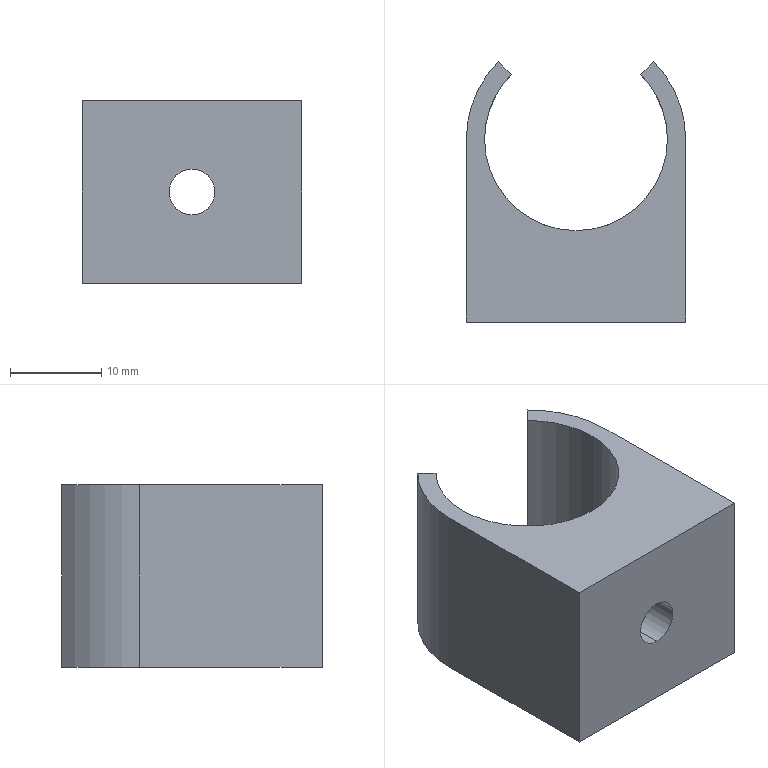Part | SolidWorks | features Extrusion 1, HoleWzd 1, ICE 1 | 1 solid | 21 faces | box 24 x 28.485 x 20 mm | volume 6832 mm3 | plane 14 | cylinder 7 | commonest cylinder face diameters 20 x3 5 x2 24 x2
STEP:
#1=CARTESIAN_POINT('',(0.,5.,7.5));
#2=VERTEX_POINT('',#1);
#3=CARTESIAN_POINT('',(0.,5.,12.5));
#4=VERTEX_POINT('',#3);
#5=CARTESIAN_POINT('',(0.,5.,10.));
#6=DIRECTION('',(0.,1.,0.));
#7=DIRECTION('',(0.,0.,-1.));
#8=AXIS2_PLACEMENT_3D('',#5,#6,#7);
#9=CIRCLE('',#8,2.5);
#10=EDGE_CURVE('',#2,#4,#9,.T.);
#11=ORIENTED_EDGE('',*,*,#10,.T.);
#12=CARTESIAN_POINT('',(0.,0.,12.5));
#13=VERTEX_POINT('',#12);
#14=CARTESIAN_POINT('',(0.,0.,12.5));
#15=DIRECTION('',(0.,-1.,0.));
#16=VECTOR('',#15,1000.);
#17=LINE('',#14,#16);
#18=EDGE_CURVE('',#4,#13,#17,.T.);
#19=ORIENTED_EDGE('',*,*,#18,.T.);
#20=CARTESIAN_POINT('',(0.,0.,7.5));
#21=VERTEX_POINT('',#20);
#22=CARTESIAN_POINT('',(0.,0.,10.));
#23=DIRECTION('',(0.,-1.,0.));
#24=DIRECTION('',(0.,0.,-1.));
#25=AXIS2_PLACEMENT_3D('',#22,#23,#24);
#26=CIRCLE('',#25,2.5);
#27=EDGE_CURVE('',#13,#21,#26,.T.);
#28=ORIENTED_EDGE('',*,*,#27,.T.);
#29=CARTESIAN_POINT('',(0.,0.,7.5));
#30=DIRECTION('',(0.,-1.,0.));
#31=VECTOR('',#30,1000.);
#32=LINE('',#29,#31);
#33=EDGE_CURVE('',#2,#21,#32,.T.);
#34=ORIENTED_EDGE('',*,*,#33,.F.);
#35=EDGE_LOOP('',(#11,#19,#28,#34));
#36=FACE_OUTER_BOUND('',#35,.T.);
#37=CARTESIAN_POINT('',(0.,0.,10.));
#38=DIRECTION('',(0.,-1.,0.));
#39=DIRECTION('',(0.,0.,-1.));
#40=AXIS2_PLACEMENT_3D('',#37,#38,#39);
#41=CYLINDRICAL_SURFACE('',#40,2.5);
#42=ADVANCED_FACE('',(#36),#41,.F.);
#43=CARTESIAN_POINT('',(2.021,10.206,6.5));
#44=VERTEX_POINT('',#43);
#45=CARTESIAN_POINT('',(-2.021,10.206,6.5));
#46=VERTEX_POINT('',#45);
#47=CARTESIAN_POINT('',(0.,20.,6.5));
#48=DIRECTION('',(0.,0.,-1.));
#49=DIRECTION('',(1.,0.,0.));
#50=AXIS2_PLACEMENT_3D('',#47,#48,#49);
#51=CIRCLE('',#50,10.);
#52=EDGE_CURVE('',#44,#46,#51,.T.);
#53=ORIENTED_EDGE('',*,*,#52,.F.);
#54=CARTESIAN_POINT('',(4.041,10.853,10.));
#55=VERTEX_POINT('',#54);
#56=CARTESIAN_POINT('',(4.041,10.853,10.));
#57=CARTESIAN_POINT('',(3.392,10.566,8.875));
#58=CARTESIAN_POINT('',(2.716,10.35,7.704));
#59=CARTESIAN_POINT('',(2.021,10.206,6.5));
#60=(BOUNDED_CURVE()B_SPLINE_CURVE(3,(#56,#57,#58,#59),.UNSPECIFIED.,.F.,.F.)B_SPLINE_CURVE_WITH_KNOTS((4,4),(4.296,4.509),.UNSPECIFIED.)CURVE()GEOMETRIC_REPRESENTATION_ITEM()RATIONAL_B_SPLINE_CURVE((1.,0.9962,0.9962,1.))REPRESENTATION_ITEM(''));
#61=EDGE_CURVE('',#55,#44,#60,.T.);
#62=ORIENTED_EDGE('',*,*,#61,.F.);
#63=CARTESIAN_POINT('',(2.021,10.206,13.5));
#64=VERTEX_POINT('',#63);
#65=CARTESIAN_POINT('',(2.021,10.206,13.5));
#66=CARTESIAN_POINT('',(2.716,10.35,12.296));
#67=CARTESIAN_POINT('',(3.392,10.566,11.125));
#68=CARTESIAN_POINT('',(4.041,10.853,10.));
#69=(BOUNDED_CURVE()B_SPLINE_CURVE(3,(#65,#66,#67,#68),.UNSPECIFIED.,.F.,.F.)B_SPLINE_CURVE_WITH_KNOTS((4,4),(4.916,5.128),.UNSPECIFIED.)CURVE()GEOMETRIC_REPRESENTATION_ITEM()RATIONAL_B_SPLINE_CURVE((1.,0.9962,0.9962,1.))REPRESENTATION_ITEM(''));
#70=EDGE_CURVE('',#64,#55,#69,.T.);
#71=ORIENTED_EDGE('',*,*,#70,.F.);
#72=CARTESIAN_POINT('',(-2.021,10.206,13.5));
#73=VERTEX_POINT('',#72);
#74=CARTESIAN_POINT('',(0.,20.,13.5));
#75=DIRECTION('',(0.,0.,1.));
#76=DIRECTION('',(-1.,0.,0.));
#77=AXIS2_PLACEMENT_3D('',#74,#75,#76);
#78=CIRCLE('',#77,10.);
#79=EDGE_CURVE('',#73,#64,#78,.T.);
#80=ORIENTED_EDGE('',*,*,#79,.F.);
#81=CARTESIAN_POINT('',(-4.041,10.853,10.));
#82=VERTEX_POINT('',#81);
#83=CARTESIAN_POINT('',(-4.041,10.853,10.));
#84=CARTESIAN_POINT('',(-3.392,10.566,11.125));
#85=CARTESIAN_POINT('',(-2.716,10.35,12.296));
#86=CARTESIAN_POINT('',(-2.021,10.206,13.5));
#87=(BOUNDED_CURVE()B_SPLINE_CURVE(3,(#83,#84,#85,#86),.UNSPECIFIED.,.F.,.F.)B_SPLINE_CURVE_WITH_KNOTS((4,4),(1.155,1.367),.UNSPECIFIED.)CURVE()GEOMETRIC_REPRESENTATION_ITEM()RATIONAL_B_SPLINE_CURVE((1.,0.9962,0.9962,1.))REPRESENTATION_ITEM(''));
#88=EDGE_CURVE('',#82,#73,#87,.T.);
#89=ORIENTED_EDGE('',*,*,#88,.F.);
#90=CARTESIAN_POINT('',(-2.021,10.206,6.5));
#91=CARTESIAN_POINT('',(-2.716,10.35,7.704));
#92=CARTESIAN_POINT('',(-3.392,10.566,8.875));
#93=CARTESIAN_POINT('',(-4.041,10.853,10.));
#94=(BOUNDED_CURVE()B_SPLINE_CURVE(3,(#90,#91,#92,#93),.UNSPECIFIED.,.F.,.F.)B_SPLINE_CURVE_WITH_KNOTS((4,4),(1.774,1.987),.UNSPECIFIED.)CURVE()GEOMETRIC_REPRESENTATION_ITEM()RATIONAL_B_SPLINE_CURVE((1.,0.9962,0.9962,1.))REPRESENTATION_ITEM(''));
#95=EDGE_CURVE('',#46,#82,#94,.T.);
#96=ORIENTED_EDGE('',*,*,#95,.F.);
#97=EDGE_LOOP('',(#53,#62,#71,#80,#89,#96));
#98=FACE_BOUND('',#97,.T.);
#99=CARTESIAN_POINT('',(10.,20.,20.));
#100=VERTEX_POINT('',#99);
#101=CARTESIAN_POINT('',(-10.,20.,20.));
#102=VERTEX_POINT('',#101);
#103=CARTESIAN_POINT('',(0.,20.,20.));
#104=DIRECTION('',(0.,0.,-1.));
#105=DIRECTION('',(1.,0.,0.));
#106=AXIS2_PLACEMENT_3D('',#103,#104,#105);
#107=CIRCLE('',#106,10.);
#108=EDGE_CURVE('',#100,#102,#107,.T.);
#109=ORIENTED_EDGE('',*,*,#108,.F.);
#110=CARTESIAN_POINT('',(10.,20.,0.));
#111=VERTEX_POINT('',#110);
#112=CARTESIAN_POINT('',(10.,20.,20.));
#113=DIRECTION('',(0.,0.,-1.));
#114=VECTOR('',#113,1000.);
#115=LINE('',#112,#114);
#116=EDGE_CURVE('',#100,#111,#115,.T.);
#117=ORIENTED_EDGE('',*,*,#116,.T.);
#118=CARTESIAN_POINT('',(-10.,20.,0.));
#119=VERTEX_POINT('',#118);
#120=CARTESIAN_POINT('',(0.,20.,0.));
#121=DIRECTION('',(0.,0.,-1.));
#122=DIRECTION('',(1.,0.,0.));
#123=AXIS2_PLACEMENT_3D('',#120,#121,#122);
#124=CIRCLE('',#123,10.);
#125=EDGE_CURVE('',#111,#119,#124,.T.);
#126=ORIENTED_EDGE('',*,*,#125,.T.);
#127=CARTESIAN_POINT('',(-10.,20.,20.));
#128=DIRECTION('',(0.,0.,-1.));
#129=VECTOR('',#128,1000.);
#130=LINE('',#127,#129);
#131=EDGE_CURVE('',#102,#119,#130,.T.);
#132=ORIENTED_EDGE('',*,*,#131,.F.);
#133=EDGE_LOOP('',(#109,#117,#126,#132));
#134=FACE_OUTER_BOUND('',#133,.T.);
#135=CARTESIAN_POINT('',(0.,20.,20.));
#136=DIRECTION('',(0.,0.,-1.));
#137=DIRECTION('',(-1.,0.,0.));
#138=AXIS2_PLACEMENT_3D('',#135,#136,#137);
#139=CYLINDRICAL_SURFACE('',#138,10.);
#140=ADVANCED_FACE('',(#98,#134),#139,.F.);
#141=CARTESIAN_POINT('',(-7.071,27.071,20.));
#142=VERTEX_POINT('',#141);
#143=CARTESIAN_POINT('',(0.,20.,20.));
#144=DIRECTION('',(0.,0.,-1.));
#145=DIRECTION('',(1.,0.,0.));
#146=AXIS2_PLACEMENT_3D('',#143,#144,#145);
#147=CIRCLE('',#146,10.);
#148=EDGE_CURVE('',#102,#142,#147,.T.);
#149=ORIENTED_EDGE('',*,*,#148,.F.);
#150=ORIENTED_EDGE('',*,*,#131,.T.);
#151=CARTESIAN_POINT('',(-7.071,27.071,0.));
#152=VERTEX_POINT('',#151);
#153=CARTESIAN_POINT('',(0.,20.,0.));
#154=DIRECTION('',(0.,0.,-1.));
#155=DIRECTION('',(1.,0.,0.));
#156=AXIS2_PLACEMENT_3D('',#153,#154,#155);
#157=CIRCLE('',#156,10.);
#158=EDGE_CURVE('',#119,#152,#157,.T.);
#159=ORIENTED_EDGE('',*,*,#158,.T.);
#160=CARTESIAN_POINT('',(-7.071,27.071,20.));
#161=DIRECTION('',(0.,0.,-1.));
#162=VECTOR('',#161,1000.);
#163=LINE('',#160,#162);
#164=EDGE_CURVE('',#142,#152,#163,.T.);
#165=ORIENTED_EDGE('',*,*,#164,.F.);
#166=EDGE_LOOP('',(#149,#150,#159,#165));
#167=FACE_OUTER_BOUND('',#166,.T.);
#168=CARTESIAN_POINT('',(0.,20.,20.));
#169=DIRECTION('',(0.,0.,-1.));
#170=DIRECTION('',(-1.,0.,0.));
#171=AXIS2_PLACEMENT_3D('',#168,#169,#170);
#172=CYLINDRICAL_SURFACE('',#171,10.);
#173=ADVANCED_FACE('',(#167),#172,.F.);
#174=ORIENTED_EDGE('',*,*,#116,.F.);
#175=CARTESIAN_POINT('',(7.071,27.071,20.));
#176=VERTEX_POINT('',#175);
#177=CARTESIAN_POINT('',(0.,20.,20.));
#178=DIRECTION('',(0.,0.,-1.));
#179=DIRECTION('',(1.,0.,0.));
#180=AXIS2_PLACEMENT_3D('',#177,#178,#179);
#181=CIRCLE('',#180,10.);
#182=EDGE_CURVE('',#176,#100,#181,.T.);
#183=ORIENTED_EDGE('',*,*,#182,.F.);
#184=CARTESIAN_POINT('',(7.071,27.071,0.));
#185=VERTEX_POINT('',#184);
#186=CARTESIAN_POINT('',(7.071,27.071,20.));
#187=DIRECTION('',(0.,0.,-1.));
#188=VECTOR('',#187,1000.);
#189=LINE('',#186,#188);
#190=EDGE_CURVE('',#176,#185,#189,.T.);
#191=ORIENTED_EDGE('',*,*,#190,.T.);
#192=CARTESIAN_POINT('',(0.,20.,0.));
#193=DIRECTION('',(0.,0.,-1.));
#194=DIRECTION('',(1.,0.,0.));
#195=AXIS2_PLACEMENT_3D('',#192,#193,#194);
#196=CIRCLE('',#195,10.);
#197=EDGE_CURVE('',#185,#111,#196,.T.);
#198=ORIENTED_EDGE('',*,*,#197,.T.);
#199=EDGE_LOOP('',(#174,#183,#191,#198));
#200=FACE_OUTER_BOUND('',#199,.T.);
#201=CARTESIAN_POINT('',(0.,20.,20.));
#202=DIRECTION('',(0.,0.,-1.));
#203=DIRECTION('',(-1.,0.,0.));
#204=AXIS2_PLACEMENT_3D('',#201,#202,#203);
#205=CYLINDRICAL_SURFACE('',#204,10.);
#206=ADVANCED_FACE('',(#200),#205,.F.);
#207=CARTESIAN_POINT('',(0.,0.,10.));
#208=DIRECTION('',(0.,-1.,0.));
#209=DIRECTION('',(0.,0.,-1.));
#210=AXIS2_PLACEMENT_3D('',#207,#208,#209);
#211=CIRCLE('',#210,2.5);
#212=EDGE_CURVE('',#21,#13,#211,.T.);
#213=ORIENTED_EDGE('',*,*,#212,.F.);
#214=ORIENTED_EDGE('',*,*,#27,.F.);
#215=EDGE_LOOP('',(#213,#214));
#216=FACE_BOUND('',#215,.T.);
#217=CARTESIAN_POINT('',(-12.,0.,0.));
#218=VERTEX_POINT('',#217);
#219=CARTESIAN_POINT('',(12.,0.,0.));
#220=VERTEX_POINT('',#219);
#221=CARTESIAN_POINT('',(-12.,0.,0.));
#222=DIRECTION('',(1.,0.,0.));
#223=VECTOR('',#222,1000.);
#224=LINE('',#221,#223);
#225=EDGE_CURVE('',#218,#220,#224,.T.);
#226=ORIENTED_EDGE('',*,*,#225,.T.);
#227=CARTESIAN_POINT('',(12.,0.,20.));
#228=VERTEX_POINT('',#227);
#229=CARTESIAN_POINT('',(12.,0.,20.));
#230=DIRECTION('',(0.,0.,-1.));
#231=VECTOR('',#230,1000.);
#232=LINE('',#229,#231);
#233=EDGE_CURVE('',#228,#220,#232,.T.);
#234=ORIENTED_EDGE('',*,*,#233,.F.);
#235=CARTESIAN_POINT('',(-12.,0.,20.));
#236=VERTEX_POINT('',#235);
#237=CARTESIAN_POINT('',(-12.,0.,20.));
#238=DIRECTION('',(1.,0.,0.));
#239=VECTOR('',#238,1000.);
#240=LINE('',#237,#239);
#241=EDGE_CURVE('',#236,#228,#240,.T.);
#242=ORIENTED_EDGE('',*,*,#241,.F.);
#243=CARTESIAN_POINT('',(-12.,0.,20.));
#244=DIRECTION('',(0.,0.,-1.));
#245=VECTOR('',#244,1000.);
#246=LINE('',#243,#245);
#247=EDGE_CURVE('',#236,#218,#246,.T.);
#248=ORIENTED_EDGE('',*,*,#247,.T.);
#249=EDGE_LOOP('',(#226,#234,#242,#248));
#250=FACE_OUTER_BOUND('',#249,.T.);
#251=CARTESIAN_POINT('',(-12.,0.,20.));
#252=DIRECTION('',(0.,1.,0.));
#253=DIRECTION('',(0.,0.,1.));
#254=AXIS2_PLACEMENT_3D('',#251,#252,#253);
#255=PLANE('',#254);
#256=ADVANCED_FACE('',(#216,#250),#255,.F.);
#257=CARTESIAN_POINT('',(12.,20.,0.));
#258=VERTEX_POINT('',#257);
#259=CARTESIAN_POINT('',(12.,10.,0.));
#260=DIRECTION('',(0.,1.,0.));
#261=VECTOR('',#260,1000.);
#262=LINE('',#259,#261);
#263=EDGE_CURVE('',#220,#258,#262,.T.);
#264=ORIENTED_EDGE('',*,*,#263,.T.);
#265=CARTESIAN_POINT('',(12.,20.,20.));
#266=VERTEX_POINT('',#265);
#267=CARTESIAN_POINT('',(12.,20.,20.));
#268=DIRECTION('',(0.,0.,-1.));
#269=VECTOR('',#268,1000.);
#270=LINE('',#267,#269);
#271=EDGE_CURVE('',#266,#258,#270,.T.);
#272=ORIENTED_EDGE('',*,*,#271,.F.);
#273=CARTESIAN_POINT('',(12.,10.,20.));
#274=DIRECTION('',(0.,1.,0.));
#275=VECTOR('',#274,1000.);
#276=LINE('',#273,#275);
#277=EDGE_CURVE('',#228,#266,#276,.T.);
#278=ORIENTED_EDGE('',*,*,#277,.F.);
#279=ORIENTED_EDGE('',*,*,#233,.T.);
#280=EDGE_LOOP('',(#264,#272,#278,#279));
#281=FACE_OUTER_BOUND('',#280,.T.);
#282=CARTESIAN_POINT('',(12.,10.,20.));
#283=DIRECTION('',(-1.,0.,0.));
#284=DIRECTION('',(0.,0.,1.));
#285=AXIS2_PLACEMENT_3D('',#282,#283,#284);
#286=PLANE('',#285);
#287=ADVANCED_FACE('',(#281),#286,.F.);
#288=CARTESIAN_POINT('',(8.485,28.485,0.));
#289=VERTEX_POINT('',#288);
#290=CARTESIAN_POINT('',(0.,20.,0.));
#291=DIRECTION('',(0.,0.,1.));
#292=DIRECTION('',(1.,0.,0.));
#293=AXIS2_PLACEMENT_3D('',#290,#291,#292);
#294=CIRCLE('',#293,12.);
#295=EDGE_CURVE('',#258,#289,#294,.T.);
#296=ORIENTED_EDGE('',*,*,#295,.T.);
#297=CARTESIAN_POINT('',(8.485,28.485,20.));
#298=VERTEX_POINT('',#297);
#299=CARTESIAN_POINT('',(8.485,28.485,20.));
#300=DIRECTION('',(0.,0.,-1.));
#301=VECTOR('',#300,1000.);
#302=LINE('',#299,#301);
#303=EDGE_CURVE('',#298,#289,#302,.T.);
#304=ORIENTED_EDGE('',*,*,#303,.F.);
#305=CARTESIAN_POINT('',(0.,20.,20.));
#306=DIRECTION('',(0.,0.,1.));
#307=DIRECTION('',(1.,0.,0.));
#308=AXIS2_PLACEMENT_3D('',#305,#306,#307);
#309=CIRCLE('',#308,12.);
#310=EDGE_CURVE('',#266,#298,#309,.T.);
#311=ORIENTED_EDGE('',*,*,#310,.F.);
#312=ORIENTED_EDGE('',*,*,#271,.T.);
#313=EDGE_LOOP('',(#296,#304,#311,#312));
#314=FACE_OUTER_BOUND('',#313,.T.);
#315=CARTESIAN_POINT('',(0.,20.,20.));
#316=DIRECTION('',(0.,0.,-1.));
#317=DIRECTION('',(-1.,0.,0.));
#318=AXIS2_PLACEMENT_3D('',#315,#316,#317);
#319=CYLINDRICAL_SURFACE('',#318,12.);
#320=ADVANCED_FACE('',(#314),#319,.T.);
#321=CARTESIAN_POINT('',(7.071,27.071,0.));
#322=DIRECTION('',(-0.7071,-0.7071,0.));
#323=VECTOR('',#322,1000.);
#324=LINE('',#321,#323);
#325=EDGE_CURVE('',#289,#185,#324,.T.);
#326=ORIENTED_EDGE('',*,*,#325,.T.);
#327=ORIENTED_EDGE('',*,*,#190,.F.);
#328=CARTESIAN_POINT('',(7.071,27.071,20.));
#329=DIRECTION('',(-0.7071,-0.7071,0.));
#330=VECTOR('',#329,1000.);
#331=LINE('',#328,#330);
#332=EDGE_CURVE('',#298,#176,#331,.T.);
#333=ORIENTED_EDGE('',*,*,#332,.F.);
#334=ORIENTED_EDGE('',*,*,#303,.T.);
#335=EDGE_LOOP('',(#326,#327,#333,#334));
#336=FACE_OUTER_BOUND('',#335,.T.);
#337=CARTESIAN_POINT('',(7.071,27.071,20.));
#338=DIRECTION('',(0.7071,-0.7071,0.));
#339=DIRECTION('',(0.7071,0.7071,0.));
#340=AXIS2_PLACEMENT_3D('',#337,#338,#339);
#341=PLANE('',#340);
#342=ADVANCED_FACE('',(#336),#341,.F.);
#343=CARTESIAN_POINT('',(-8.485,28.485,0.));
#344=VERTEX_POINT('',#343);
#345=CARTESIAN_POINT('',(-7.071,27.071,0.));
#346=DIRECTION('',(-0.7071,0.7071,0.));
#347=VECTOR('',#346,1000.);
#348=LINE('',#345,#347);
#349=EDGE_CURVE('',#152,#344,#348,.T.);
#350=ORIENTED_EDGE('',*,*,#349,.T.);
#351=CARTESIAN_POINT('',(-8.485,28.485,20.));
#352=VERTEX_POINT('',#351);
#353=CARTESIAN_POINT('',(-8.485,28.485,20.));
#354=DIRECTION('',(0.,0.,-1.));
#355=VECTOR('',#354,1000.);
#356=LINE('',#353,#355);
#357=EDGE_CURVE('',#352,#344,#356,.T.);
#358=ORIENTED_EDGE('',*,*,#357,.F.);
#359=CARTESIAN_POINT('',(-7.071,27.071,20.));
#360=DIRECTION('',(-0.7071,0.7071,0.));
#361=VECTOR('',#360,1000.);
#362=LINE('',#359,#361);
#363=EDGE_CURVE('',#142,#352,#362,.T.);
#364=ORIENTED_EDGE('',*,*,#363,.F.);
#365=ORIENTED_EDGE('',*,*,#164,.T.);
#366=EDGE_LOOP('',(#350,#358,#364,#365));
#367=FACE_OUTER_BOUND('',#366,.T.);
#368=CARTESIAN_POINT('',(-7.071,27.071,20.));
#369=DIRECTION('',(-0.7071,-0.7071,0.));
#370=DIRECTION('',(0.7071,-0.7071,0.));
#371=AXIS2_PLACEMENT_3D('',#368,#369,#370);
#372=PLANE('',#371);
#373=ADVANCED_FACE('',(#367),#372,.F.);
#374=CARTESIAN_POINT('',(-12.,20.,0.));
#375=VERTEX_POINT('',#374);
#376=CARTESIAN_POINT('',(0.,20.,0.));
#377=DIRECTION('',(0.,0.,1.));
#378=DIRECTION('',(1.,0.,0.));
#379=AXIS2_PLACEMENT_3D('',#376,#377,#378);
#380=CIRCLE('',#379,12.);
#381=EDGE_CURVE('',#344,#375,#380,.T.);
#382=ORIENTED_EDGE('',*,*,#381,.T.);
#383=CARTESIAN_POINT('',(-12.,20.,20.));
#384=VERTEX_POINT('',#383);
#385=CARTESIAN_POINT('',(-12.,20.,20.));
#386=DIRECTION('',(0.,0.,-1.));
#387=VECTOR('',#386,1000.);
#388=LINE('',#385,#387);
#389=EDGE_CURVE('',#384,#375,#388,.T.);
#390=ORIENTED_EDGE('',*,*,#389,.F.);
#391=CARTESIAN_POINT('',(0.,20.,20.));
#392=DIRECTION('',(0.,0.,1.));
#393=DIRECTION('',(1.,0.,0.));
#394=AXIS2_PLACEMENT_3D('',#391,#392,#393);
#395=CIRCLE('',#394,12.);
#396=EDGE_CURVE('',#352,#384,#395,.T.);
#397=ORIENTED_EDGE('',*,*,#396,.F.);
#398=ORIENTED_EDGE('',*,*,#357,.T.);
#399=EDGE_LOOP('',(#382,#390,#397,#398));
#400=FACE_OUTER_BOUND('',#399,.T.);
#401=CARTESIAN_POINT('',(0.,20.,20.));
#402=DIRECTION('',(0.,0.,-1.));
#403=DIRECTION('',(-1.,0.,0.));
#404=AXIS2_PLACEMENT_3D('',#401,#402,#403);
#405=CYLINDRICAL_SURFACE('',#404,12.);
#406=ADVANCED_FACE('',(#400),#405,.T.);
#407=CARTESIAN_POINT('',(-12.,10.,0.));
#408=DIRECTION('',(0.,-1.,0.));
#409=VECTOR('',#408,1000.);
#410=LINE('',#407,#409);
#411=EDGE_CURVE('',#375,#218,#410,.T.);
#412=ORIENTED_EDGE('',*,*,#411,.T.);
#413=ORIENTED_EDGE('',*,*,#247,.F.);
#414=CARTESIAN_POINT('',(-12.,10.,20.));
#415=DIRECTION('',(0.,-1.,0.));
#416=VECTOR('',#415,1000.);
#417=LINE('',#414,#416);
#418=EDGE_CURVE('',#384,#236,#417,.T.);
#419=ORIENTED_EDGE('',*,*,#418,.F.);
#420=ORIENTED_EDGE('',*,*,#389,.T.);
#421=EDGE_LOOP('',(#412,#413,#419,#420));
#422=FACE_OUTER_BOUND('',#421,.T.);
#423=CARTESIAN_POINT('',(-12.,10.,20.));
#424=DIRECTION('',(1.,0.,0.));
#425=DIRECTION('',(0.,0.,-1.));
#426=AXIS2_PLACEMENT_3D('',#423,#424,#425);
#427=PLANE('',#426);
#428=ADVANCED_FACE('',(#422),#427,.F.);
#429=ORIENTED_EDGE('',*,*,#418,.T.);
#430=ORIENTED_EDGE('',*,*,#241,.T.);
#431=ORIENTED_EDGE('',*,*,#277,.T.);
#432=ORIENTED_EDGE('',*,*,#310,.T.);
#433=ORIENTED_EDGE('',*,*,#332,.T.);
#434=ORIENTED_EDGE('',*,*,#182,.T.);
#435=ORIENTED_EDGE('',*,*,#108,.T.);
#436=ORIENTED_EDGE('',*,*,#148,.T.);
#437=ORIENTED_EDGE('',*,*,#363,.T.);
#438=ORIENTED_EDGE('',*,*,#396,.T.);
#439=EDGE_LOOP('',(#429,#430,#431,#432,#433,#434,#435,#436,#437,#438));
#440=FACE_OUTER_BOUND('',#439,.T.);
#441=CARTESIAN_POINT('',(0.,20.,20.));
#442=DIRECTION('',(0.,0.,1.));
#443=DIRECTION('',(1.,0.,0.));
#444=AXIS2_PLACEMENT_3D('',#441,#442,#443);
#445=PLANE('',#444);
#446=ADVANCED_FACE('',(#440),#445,.T.);
#447=ORIENTED_EDGE('',*,*,#225,.F.);
#448=ORIENTED_EDGE('',*,*,#411,.F.);
#449=ORIENTED_EDGE('',*,*,#381,.F.);
#450=ORIENTED_EDGE('',*,*,#349,.F.);
#451=ORIENTED_EDGE('',*,*,#158,.F.);
#452=ORIENTED_EDGE('',*,*,#125,.F.);
#453=ORIENTED_EDGE('',*,*,#197,.F.);
#454=ORIENTED_EDGE('',*,*,#325,.F.);
#455=ORIENTED_EDGE('',*,*,#295,.F.);
#456=ORIENTED_EDGE('',*,*,#263,.F.);
#457=EDGE_LOOP('',(#447,#448,#449,#450,#451,#452,#453,#454,#455,#456));
#458=FACE_OUTER_BOUND('',#457,.T.);
#459=CARTESIAN_POINT('',(0.,20.,0.));
#460=DIRECTION('',(0.,0.,1.));
#461=DIRECTION('',(1.,0.,0.));
#462=AXIS2_PLACEMENT_3D('',#459,#460,#461);
#463=PLANE('',#462);
#464=ADVANCED_FACE('',(#458),#463,.F.);
#465=ORIENTED_EDGE('',*,*,#18,.F.);
#466=CARTESIAN_POINT('',(0.,5.,10.));
#467=DIRECTION('',(0.,1.,0.));
#468=DIRECTION('',(0.,0.,-1.));
#469=AXIS2_PLACEMENT_3D('',#466,#467,#468);
#470=CIRCLE('',#469,2.5);
#471=EDGE_CURVE('',#4,#2,#470,.T.);
#472=ORIENTED_EDGE('',*,*,#471,.T.);
#473=ORIENTED_EDGE('',*,*,#33,.T.);
#474=ORIENTED_EDGE('',*,*,#212,.T.);
#475=EDGE_LOOP('',(#465,#472,#473,#474));
#476=FACE_OUTER_BOUND('',#475,.T.);
#477=CARTESIAN_POINT('',(0.,0.,10.));
#478=DIRECTION('',(0.,-1.,0.));
#479=DIRECTION('',(0.,0.,-1.));
#480=AXIS2_PLACEMENT_3D('',#477,#478,#479);
#481=CYLINDRICAL_SURFACE('',#480,2.5);
#482=ADVANCED_FACE('',(#476),#481,.F.);
#483=ORIENTED_EDGE('',*,*,#52,.T.);
#484=CARTESIAN_POINT('',(-2.021,5.,6.5));
#485=VERTEX_POINT('',#484);
#486=CARTESIAN_POINT('',(-2.021,5.,6.5));
#487=DIRECTION('',(0.,1.,0.));
#488=VECTOR('',#487,1000.);
#489=LINE('',#486,#488);
#490=EDGE_CURVE('',#485,#46,#489,.T.);
#491=ORIENTED_EDGE('',*,*,#490,.F.);
#492=CARTESIAN_POINT('',(2.021,5.,6.5));
#493=VERTEX_POINT('',#492);
#494=CARTESIAN_POINT('',(-2.021,5.,6.5));
#495=DIRECTION('',(1.,0.,0.));
#496=VECTOR('',#495,1000.);
#497=LINE('',#494,#496);
#498=EDGE_CURVE('',#485,#493,#497,.T.);
#499=ORIENTED_EDGE('',*,*,#498,.T.);
#500=CARTESIAN_POINT('',(2.021,5.,6.5));
#501=DIRECTION('',(0.,1.,0.));
#502=VECTOR('',#501,1000.);
#503=LINE('',#500,#502);
#504=EDGE_CURVE('',#493,#44,#503,.T.);
#505=ORIENTED_EDGE('',*,*,#504,.T.);
#506=EDGE_LOOP('',(#483,#491,#499,#505));
#507=FACE_OUTER_BOUND('',#506,.T.);
#508=CARTESIAN_POINT('',(-2.021,5.,6.5));
#509=DIRECTION('',(0.,0.,1.));
#510=DIRECTION('',(1.,0.,0.));
#511=AXIS2_PLACEMENT_3D('',#508,#509,#510);
#512=PLANE('',#511);
#513=ADVANCED_FACE('',(#507),#512,.T.);
#514=ORIENTED_EDGE('',*,*,#61,.T.);
#515=ORIENTED_EDGE('',*,*,#504,.F.);
#516=CARTESIAN_POINT('',(4.041,5.,10.));
#517=VERTEX_POINT('',#516);
#518=CARTESIAN_POINT('',(2.021,5.,6.5));
#519=DIRECTION('',(0.5,0.,0.866));
#520=VECTOR('',#519,1000.);
#521=LINE('',#518,#520);
#522=EDGE_CURVE('',#493,#517,#521,.T.);
#523=ORIENTED_EDGE('',*,*,#522,.T.);
#524=CARTESIAN_POINT('',(4.041,5.,10.));
#525=DIRECTION('',(0.,1.,0.));
#526=VECTOR('',#525,1000.);
#527=LINE('',#524,#526);
#528=EDGE_CURVE('',#517,#55,#527,.T.);
#529=ORIENTED_EDGE('',*,*,#528,.T.);
#530=EDGE_LOOP('',(#514,#515,#523,#529));
#531=FACE_OUTER_BOUND('',#530,.T.);
#532=CARTESIAN_POINT('',(2.021,5.,6.5));
#533=DIRECTION('',(-0.866,0.,0.5));
#534=DIRECTION('',(0.5,0.,0.866));
#535=AXIS2_PLACEMENT_3D('',#532,#533,#534);
#536=PLANE('',#535);
#537=ADVANCED_FACE('',(#531),#536,.T.);
#538=ORIENTED_EDGE('',*,*,#70,.T.);
#539=ORIENTED_EDGE('',*,*,#528,.F.);
#540=CARTESIAN_POINT('',(2.021,5.,13.5));
#541=VERTEX_POINT('',#540);
#542=CARTESIAN_POINT('',(4.041,5.,10.));
#543=DIRECTION('',(-0.5,0.,0.866));
#544=VECTOR('',#543,1000.);
#545=LINE('',#542,#544);
#546=EDGE_CURVE('',#517,#541,#545,.T.);
#547=ORIENTED_EDGE('',*,*,#546,.T.);
#548=CARTESIAN_POINT('',(2.021,5.,13.5));
#549=DIRECTION('',(0.,1.,0.));
#550=VECTOR('',#549,1000.);
#551=LINE('',#548,#550);
#552=EDGE_CURVE('',#541,#64,#551,.T.);
#553=ORIENTED_EDGE('',*,*,#552,.T.);
#554=EDGE_LOOP('',(#538,#539,#547,#553));
#555=FACE_OUTER_BOUND('',#554,.T.);
#556=CARTESIAN_POINT('',(4.041,5.,10.));
#557=DIRECTION('',(-0.866,0.,-0.5));
#558=DIRECTION('',(-0.5,0.,0.866));
#559=AXIS2_PLACEMENT_3D('',#556,#557,#558);
#560=PLANE('',#559);
#561=ADVANCED_FACE('',(#555),#560,.T.);
#562=ORIENTED_EDGE('',*,*,#79,.T.);
#563=ORIENTED_EDGE('',*,*,#552,.F.);
#564=CARTESIAN_POINT('',(-2.021,5.,13.5));
#565=VERTEX_POINT('',#564);
#566=CARTESIAN_POINT('',(2.021,5.,13.5));
#567=DIRECTION('',(-1.,0.,0.));
#568=VECTOR('',#567,1000.);
#569=LINE('',#566,#568);
#570=EDGE_CURVE('',#541,#565,#569,.T.);
#571=ORIENTED_EDGE('',*,*,#570,.T.);
#572=CARTESIAN_POINT('',(-2.021,5.,13.5));
#573=DIRECTION('',(0.,1.,0.));
#574=VECTOR('',#573,1000.);
#575=LINE('',#572,#574);
#576=EDGE_CURVE('',#565,#73,#575,.T.);
#577=ORIENTED_EDGE('',*,*,#576,.T.);
#578=EDGE_LOOP('',(#562,#563,#571,#577));
#579=FACE_OUTER_BOUND('',#578,.T.);
#580=CARTESIAN_POINT('',(2.021,5.,13.5));
#581=DIRECTION('',(0.,0.,-1.));
#582=DIRECTION('',(-1.,0.,0.));
#583=AXIS2_PLACEMENT_3D('',#580,#581,#582);
#584=PLANE('',#583);
#585=ADVANCED_FACE('',(#579),#584,.T.);
#586=ORIENTED_EDGE('',*,*,#88,.T.);
#587=ORIENTED_EDGE('',*,*,#576,.F.);
#588=CARTESIAN_POINT('',(-4.041,5.,10.));
#589=VERTEX_POINT('',#588);
#590=CARTESIAN_POINT('',(-2.021,5.,13.5));
#591=DIRECTION('',(-0.5,0.,-0.866));
#592=VECTOR('',#591,1000.);
#593=LINE('',#590,#592);
#594=EDGE_CURVE('',#565,#589,#593,.T.);
#595=ORIENTED_EDGE('',*,*,#594,.T.);
#596=CARTESIAN_POINT('',(-4.041,5.,10.));
#597=DIRECTION('',(0.,1.,0.));
#598=VECTOR('',#597,1000.);
#599=LINE('',#596,#598);
#600=EDGE_CURVE('',#589,#82,#599,.T.);
#601=ORIENTED_EDGE('',*,*,#600,.T.);
#602=EDGE_LOOP('',(#586,#587,#595,#601));
#603=FACE_OUTER_BOUND('',#602,.T.);
#604=CARTESIAN_POINT('',(-2.021,5.,13.5));
#605=DIRECTION('',(0.866,0.,-0.5));
#606=DIRECTION('',(-0.5,0.,-0.866));
#607=AXIS2_PLACEMENT_3D('',#604,#605,#606);
#608=PLANE('',#607);
#609=ADVANCED_FACE('',(#603),#608,.T.);
#610=ORIENTED_EDGE('',*,*,#95,.T.);
#611=ORIENTED_EDGE('',*,*,#600,.F.);
#612=CARTESIAN_POINT('',(-4.041,5.,10.));
#613=DIRECTION('',(0.5,0.,-0.866));
#614=VECTOR('',#613,1000.);
#615=LINE('',#612,#614);
#616=EDGE_CURVE('',#589,#485,#615,.T.);
#617=ORIENTED_EDGE('',*,*,#616,.T.);
#618=ORIENTED_EDGE('',*,*,#490,.T.);
#619=EDGE_LOOP('',(#610,#611,#617,#618));
#620=FACE_OUTER_BOUND('',#619,.T.);
#621=CARTESIAN_POINT('',(-4.041,5.,10.));
#622=DIRECTION('',(0.866,0.,0.5));
#623=DIRECTION('',(0.5,0.,-0.866));
#624=AXIS2_PLACEMENT_3D('',#621,#622,#623);
#625=PLANE('',#624);
#626=ADVANCED_FACE('',(#620),#625,.T.);
#627=ORIENTED_EDGE('',*,*,#498,.F.);
#628=ORIENTED_EDGE('',*,*,#616,.F.);
#629=ORIENTED_EDGE('',*,*,#594,.F.);
#630=ORIENTED_EDGE('',*,*,#570,.F.);
#631=ORIENTED_EDGE('',*,*,#546,.F.);
#632=ORIENTED_EDGE('',*,*,#522,.F.);
#633=EDGE_LOOP('',(#627,#628,#629,#630,#631,#632));
#634=FACE_OUTER_BOUND('',#633,.T.);
#635=ORIENTED_EDGE('',*,*,#10,.F.);
#636=ORIENTED_EDGE('',*,*,#471,.F.);
#637=EDGE_LOOP('',(#635,#636));
#638=FACE_BOUND('',#637,.T.);
#639=CARTESIAN_POINT('',(0.,5.,0.));
#640=DIRECTION('',(0.,-1.,0.));
#641=DIRECTION('',(0.,0.,-1.));
#642=AXIS2_PLACEMENT_3D('',#639,#640,#641);
#643=PLANE('',#642);
#644=ADVANCED_FACE('',(#634,#638),#643,.F.);
#645=CLOSED_SHELL('',(#42,#140,#173,#206,#256,#287,#320,#342,#373,#406,#428,#446,#464,#482,#513,#537,#561,#585,#609,#626,#644));
#646=MANIFOLD_SOLID_BREP('',#645);
#647=CARTESIAN_POINT('',(0.,0.,0.));
#648=DIRECTION('',(0.,0.,1.));
#649=DIRECTION('',(1.,0.,0.));
#650=AXIS2_PLACEMENT_3D('',#647,#648,#649);
#651=(LENGTH_UNIT()NAMED_UNIT(*)SI_UNIT(.MILLI.,.METRE.));
#652=UNCERTAINTY_MEASURE_WITH_UNIT(LENGTH_MEASURE(0.00001),#651,'','');
#653=(NAMED_UNIT(*)PLANE_ANGLE_UNIT()SI_UNIT($,.RADIAN.));
#654=(NAMED_UNIT(*)SI_UNIT($,.STERADIAN.)SOLID_ANGLE_UNIT());
#655=(GEOMETRIC_REPRESENTATION_CONTEXT(3)GLOBAL_UNCERTAINTY_ASSIGNED_CONTEXT((#652))GLOBAL_UNIT_ASSIGNED_CONTEXT((#651,#653,#654))REPRESENTATION_CONTEXT('',''));
#656=ADVANCED_BREP_SHAPE_REPRESENTATION('',(#646,#650),#655);